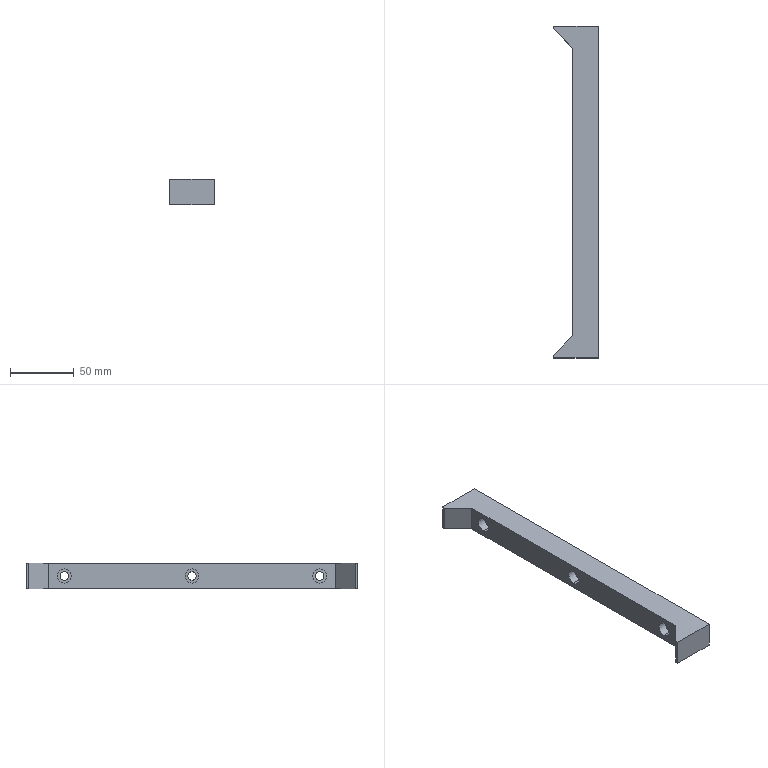Part | STEP file | X77-03204g | 1 solid | 25 faces | box 35 x 260 x 20 mm | volume 106557 mm3 | plane 13 | cylinder 12 | commonest cylinder face diameters 6.6 x6 11 x6
STEP:
#1=CARTESIAN_POINT('',(-11.074,-15.,-15.5));
#2=VERTEX_POINT('',#1);
#3=CARTESIAN_POINT('',(-11.074,-15.,-4.5));
#4=VERTEX_POINT('',#3);
#5=CARTESIAN_POINT('',(-11.074,-15.,-10.));
#6=DIRECTION('',(-1.,0.,0.));
#7=DIRECTION('',(0.,0.,1.));
#8=AXIS2_PLACEMENT_3D('',#5,#6,#7);
#9=CIRCLE('',#8,5.5);
#10=EDGE_CURVE('',#2,#4,#9,.T.);
#11=ORIENTED_EDGE('',*,*,#10,.F.);
#12=CARTESIAN_POINT('',(-17.874,-15.,-15.5));
#13=VERTEX_POINT('',#12);
#14=CARTESIAN_POINT('',(-17.874,-15.,-15.5));
#15=DIRECTION('',(-1.,0.,0.));
#16=VECTOR('',#15,1000.);
#17=LINE('',#14,#16);
#18=EDGE_CURVE('',#2,#13,#17,.T.);
#19=ORIENTED_EDGE('',*,*,#18,.T.);
#20=CARTESIAN_POINT('',(-17.874,-15.,-4.5));
#21=VERTEX_POINT('',#20);
#22=CARTESIAN_POINT('',(-17.874,-15.,-10.));
#23=DIRECTION('',(-1.,0.,0.));
#24=DIRECTION('',(0.,0.,1.));
#25=AXIS2_PLACEMENT_3D('',#22,#23,#24);
#26=CIRCLE('',#25,5.5);
#27=EDGE_CURVE('',#13,#21,#26,.T.);
#28=ORIENTED_EDGE('',*,*,#27,.T.);
#29=CARTESIAN_POINT('',(-17.874,-15.,-4.5));
#30=DIRECTION('',(-1.,0.,0.));
#31=VECTOR('',#30,1000.);
#32=LINE('',#29,#31);
#33=EDGE_CURVE('',#4,#21,#32,.T.);
#34=ORIENTED_EDGE('',*,*,#33,.F.);
#35=EDGE_LOOP('',(#11,#19,#28,#34));
#36=FACE_OUTER_BOUND('',#35,.T.);
#37=CARTESIAN_POINT('',(-17.874,-15.,-10.));
#38=DIRECTION('',(-1.,0.,0.));
#39=DIRECTION('',(0.,0.,1.));
#40=AXIS2_PLACEMENT_3D('',#37,#38,#39);
#41=CYLINDRICAL_SURFACE('',#40,5.5);
#42=ADVANCED_FACE('',(#36),#41,.F.);
#43=CARTESIAN_POINT('',(2.126,-15.,-13.3));
#44=VERTEX_POINT('',#43);
#45=CARTESIAN_POINT('',(2.126,-15.,-6.7));
#46=VERTEX_POINT('',#45);
#47=CARTESIAN_POINT('',(2.126,-15.,-10.));
#48=DIRECTION('',(-1.,0.,0.));
#49=DIRECTION('',(0.,0.,1.));
#50=AXIS2_PLACEMENT_3D('',#47,#48,#49);
#51=CIRCLE('',#50,3.3);
#52=EDGE_CURVE('',#44,#46,#51,.T.);
#53=ORIENTED_EDGE('',*,*,#52,.F.);
#54=CARTESIAN_POINT('',(-11.074,-15.,-13.3));
#55=VERTEX_POINT('',#54);
#56=CARTESIAN_POINT('',(-17.874,-15.,-13.3));
#57=DIRECTION('',(-1.,0.,0.));
#58=VECTOR('',#57,1000.);
#59=LINE('',#56,#58);
#60=EDGE_CURVE('',#44,#55,#59,.T.);
#61=ORIENTED_EDGE('',*,*,#60,.T.);
#62=CARTESIAN_POINT('',(-11.074,-15.,-6.7));
#63=VERTEX_POINT('',#62);
#64=CARTESIAN_POINT('',(-11.074,-15.,-10.));
#65=DIRECTION('',(-1.,0.,0.));
#66=DIRECTION('',(0.,0.,1.));
#67=AXIS2_PLACEMENT_3D('',#64,#65,#66);
#68=CIRCLE('',#67,3.3);
#69=EDGE_CURVE('',#55,#63,#68,.T.);
#70=ORIENTED_EDGE('',*,*,#69,.T.);
#71=CARTESIAN_POINT('',(-17.874,-15.,-6.7));
#72=DIRECTION('',(-1.,0.,0.));
#73=VECTOR('',#72,1000.);
#74=LINE('',#71,#73);
#75=EDGE_CURVE('',#46,#63,#74,.T.);
#76=ORIENTED_EDGE('',*,*,#75,.F.);
#77=EDGE_LOOP('',(#53,#61,#70,#76));
#78=FACE_OUTER_BOUND('',#77,.T.);
#79=CARTESIAN_POINT('',(-17.874,-15.,-10.));
#80=DIRECTION('',(-1.,0.,0.));
#81=DIRECTION('',(0.,0.,1.));
#82=AXIS2_PLACEMENT_3D('',#79,#80,#81);
#83=CYLINDRICAL_SURFACE('',#82,3.3);
#84=ADVANCED_FACE('',(#78),#83,.F.);
#85=CARTESIAN_POINT('',(-11.074,-115.,-15.5));
#86=VERTEX_POINT('',#85);
#87=CARTESIAN_POINT('',(-11.074,-115.,-4.5));
#88=VERTEX_POINT('',#87);
#89=CARTESIAN_POINT('',(-11.074,-115.,-10.));
#90=DIRECTION('',(-1.,0.,0.));
#91=DIRECTION('',(0.,0.,1.));
#92=AXIS2_PLACEMENT_3D('',#89,#90,#91);
#93=CIRCLE('',#92,5.5);
#94=EDGE_CURVE('',#86,#88,#93,.T.);
#95=ORIENTED_EDGE('',*,*,#94,.F.);
#96=CARTESIAN_POINT('',(-17.874,-115.,-15.5));
#97=VERTEX_POINT('',#96);
#98=CARTESIAN_POINT('',(-17.874,-115.,-15.5));
#99=DIRECTION('',(-1.,0.,0.));
#100=VECTOR('',#99,1000.);
#101=LINE('',#98,#100);
#102=EDGE_CURVE('',#86,#97,#101,.T.);
#103=ORIENTED_EDGE('',*,*,#102,.T.);
#104=CARTESIAN_POINT('',(-17.874,-115.,-4.5));
#105=VERTEX_POINT('',#104);
#106=CARTESIAN_POINT('',(-17.874,-115.,-10.));
#107=DIRECTION('',(-1.,0.,0.));
#108=DIRECTION('',(0.,0.,1.));
#109=AXIS2_PLACEMENT_3D('',#106,#107,#108);
#110=CIRCLE('',#109,5.5);
#111=EDGE_CURVE('',#97,#105,#110,.T.);
#112=ORIENTED_EDGE('',*,*,#111,.T.);
#113=CARTESIAN_POINT('',(-17.874,-115.,-4.5));
#114=DIRECTION('',(-1.,0.,0.));
#115=VECTOR('',#114,1000.);
#116=LINE('',#113,#115);
#117=EDGE_CURVE('',#88,#105,#116,.T.);
#118=ORIENTED_EDGE('',*,*,#117,.F.);
#119=EDGE_LOOP('',(#95,#103,#112,#118));
#120=FACE_OUTER_BOUND('',#119,.T.);
#121=CARTESIAN_POINT('',(-17.874,-115.,-10.));
#122=DIRECTION('',(-1.,0.,0.));
#123=DIRECTION('',(0.,0.,1.));
#124=AXIS2_PLACEMENT_3D('',#121,#122,#123);
#125=CYLINDRICAL_SURFACE('',#124,5.5);
#126=ADVANCED_FACE('',(#120),#125,.F.);
#127=CARTESIAN_POINT('',(2.126,-115.,-13.3));
#128=VERTEX_POINT('',#127);
#129=CARTESIAN_POINT('',(2.126,-115.,-6.7));
#130=VERTEX_POINT('',#129);
#131=CARTESIAN_POINT('',(2.126,-115.,-10.));
#132=DIRECTION('',(-1.,0.,0.));
#133=DIRECTION('',(0.,0.,1.));
#134=AXIS2_PLACEMENT_3D('',#131,#132,#133);
#135=CIRCLE('',#134,3.3);
#136=EDGE_CURVE('',#128,#130,#135,.T.);
#137=ORIENTED_EDGE('',*,*,#136,.F.);
#138=CARTESIAN_POINT('',(-11.074,-115.,-13.3));
#139=VERTEX_POINT('',#138);
#140=CARTESIAN_POINT('',(-17.874,-115.,-13.3));
#141=DIRECTION('',(-1.,0.,0.));
#142=VECTOR('',#141,1000.);
#143=LINE('',#140,#142);
#144=EDGE_CURVE('',#128,#139,#143,.T.);
#145=ORIENTED_EDGE('',*,*,#144,.T.);
#146=CARTESIAN_POINT('',(-11.074,-115.,-6.7));
#147=VERTEX_POINT('',#146);
#148=CARTESIAN_POINT('',(-11.074,-115.,-10.));
#149=DIRECTION('',(-1.,0.,0.));
#150=DIRECTION('',(0.,0.,1.));
#151=AXIS2_PLACEMENT_3D('',#148,#149,#150);
#152=CIRCLE('',#151,3.3);
#153=EDGE_CURVE('',#139,#147,#152,.T.);
#154=ORIENTED_EDGE('',*,*,#153,.T.);
#155=CARTESIAN_POINT('',(-17.874,-115.,-6.7));
#156=DIRECTION('',(-1.,0.,0.));
#157=VECTOR('',#156,1000.);
#158=LINE('',#155,#157);
#159=EDGE_CURVE('',#130,#147,#158,.T.);
#160=ORIENTED_EDGE('',*,*,#159,.F.);
#161=EDGE_LOOP('',(#137,#145,#154,#160));
#162=FACE_OUTER_BOUND('',#161,.T.);
#163=CARTESIAN_POINT('',(-17.874,-115.,-10.));
#164=DIRECTION('',(-1.,0.,0.));
#165=DIRECTION('',(0.,0.,1.));
#166=AXIS2_PLACEMENT_3D('',#163,#164,#165);
#167=CYLINDRICAL_SURFACE('',#166,3.3);
#168=ADVANCED_FACE('',(#162),#167,.F.);
#169=CARTESIAN_POINT('',(-11.074,-215.,-15.5));
#170=VERTEX_POINT('',#169);
#171=CARTESIAN_POINT('',(-11.074,-215.,-4.5));
#172=VERTEX_POINT('',#171);
#173=CARTESIAN_POINT('',(-11.074,-215.,-10.));
#174=DIRECTION('',(-1.,0.,0.));
#175=DIRECTION('',(0.,0.,1.));
#176=AXIS2_PLACEMENT_3D('',#173,#174,#175);
#177=CIRCLE('',#176,5.5);
#178=EDGE_CURVE('',#170,#172,#177,.T.);
#179=ORIENTED_EDGE('',*,*,#178,.F.);
#180=CARTESIAN_POINT('',(-17.874,-215.,-15.5));
#181=VERTEX_POINT('',#180);
#182=CARTESIAN_POINT('',(-17.874,-215.,-15.5));
#183=DIRECTION('',(-1.,0.,0.));
#184=VECTOR('',#183,1000.);
#185=LINE('',#182,#184);
#186=EDGE_CURVE('',#170,#181,#185,.T.);
#187=ORIENTED_EDGE('',*,*,#186,.T.);
#188=CARTESIAN_POINT('',(-17.874,-215.,-4.5));
#189=VERTEX_POINT('',#188);
#190=CARTESIAN_POINT('',(-17.874,-215.,-10.));
#191=DIRECTION('',(-1.,0.,0.));
#192=DIRECTION('',(0.,0.,1.));
#193=AXIS2_PLACEMENT_3D('',#190,#191,#192);
#194=CIRCLE('',#193,5.5);
#195=EDGE_CURVE('',#181,#189,#194,.T.);
#196=ORIENTED_EDGE('',*,*,#195,.T.);
#197=CARTESIAN_POINT('',(-17.874,-215.,-4.5));
#198=DIRECTION('',(-1.,0.,0.));
#199=VECTOR('',#198,1000.);
#200=LINE('',#197,#199);
#201=EDGE_CURVE('',#172,#189,#200,.T.);
#202=ORIENTED_EDGE('',*,*,#201,.F.);
#203=EDGE_LOOP('',(#179,#187,#196,#202));
#204=FACE_OUTER_BOUND('',#203,.T.);
#205=CARTESIAN_POINT('',(-17.874,-215.,-10.));
#206=DIRECTION('',(-1.,0.,0.));
#207=DIRECTION('',(0.,0.,1.));
#208=AXIS2_PLACEMENT_3D('',#205,#206,#207);
#209=CYLINDRICAL_SURFACE('',#208,5.5);
#210=ADVANCED_FACE('',(#204),#209,.F.);
#211=CARTESIAN_POINT('',(2.126,-215.,-13.3));
#212=VERTEX_POINT('',#211);
#213=CARTESIAN_POINT('',(2.126,-215.,-6.7));
#214=VERTEX_POINT('',#213);
#215=CARTESIAN_POINT('',(2.126,-215.,-10.));
#216=DIRECTION('',(-1.,0.,0.));
#217=DIRECTION('',(0.,0.,1.));
#218=AXIS2_PLACEMENT_3D('',#215,#216,#217);
#219=CIRCLE('',#218,3.3);
#220=EDGE_CURVE('',#212,#214,#219,.T.);
#221=ORIENTED_EDGE('',*,*,#220,.F.);
#222=CARTESIAN_POINT('',(-11.074,-215.,-13.3));
#223=VERTEX_POINT('',#222);
#224=CARTESIAN_POINT('',(-17.874,-215.,-13.3));
#225=DIRECTION('',(-1.,0.,0.));
#226=VECTOR('',#225,1000.);
#227=LINE('',#224,#226);
#228=EDGE_CURVE('',#212,#223,#227,.T.);
#229=ORIENTED_EDGE('',*,*,#228,.T.);
#230=CARTESIAN_POINT('',(-11.074,-215.,-6.7));
#231=VERTEX_POINT('',#230);
#232=CARTESIAN_POINT('',(-11.074,-215.,-10.));
#233=DIRECTION('',(-1.,0.,0.));
#234=DIRECTION('',(0.,0.,1.));
#235=AXIS2_PLACEMENT_3D('',#232,#233,#234);
#236=CIRCLE('',#235,3.3);
#237=EDGE_CURVE('',#223,#231,#236,.T.);
#238=ORIENTED_EDGE('',*,*,#237,.T.);
#239=CARTESIAN_POINT('',(-17.874,-215.,-6.7));
#240=DIRECTION('',(-1.,0.,0.));
#241=VECTOR('',#240,1000.);
#242=LINE('',#239,#241);
#243=EDGE_CURVE('',#214,#231,#242,.T.);
#244=ORIENTED_EDGE('',*,*,#243,.F.);
#245=EDGE_LOOP('',(#221,#229,#238,#244));
#246=FACE_OUTER_BOUND('',#245,.T.);
#247=CARTESIAN_POINT('',(-17.874,-215.,-10.));
#248=DIRECTION('',(-1.,0.,0.));
#249=DIRECTION('',(0.,0.,1.));
#250=AXIS2_PLACEMENT_3D('',#247,#248,#249);
#251=CYLINDRICAL_SURFACE('',#250,3.3);
#252=ADVANCED_FACE('',(#246),#251,.F.);
#253=CARTESIAN_POINT('',(-17.874,-15.,-10.));
#254=DIRECTION('',(-1.,0.,0.));
#255=DIRECTION('',(0.,0.,1.));
#256=AXIS2_PLACEMENT_3D('',#253,#254,#255);
#257=CIRCLE('',#256,5.5);
#258=EDGE_CURVE('',#21,#13,#257,.T.);
#259=ORIENTED_EDGE('',*,*,#258,.F.);
#260=ORIENTED_EDGE('',*,*,#27,.F.);
#261=EDGE_LOOP('',(#259,#260));
#262=FACE_BOUND('',#261,.T.);
#263=CARTESIAN_POINT('',(-17.874,-115.,-10.));
#264=DIRECTION('',(-1.,0.,0.));
#265=DIRECTION('',(0.,0.,1.));
#266=AXIS2_PLACEMENT_3D('',#263,#264,#265);
#267=CIRCLE('',#266,5.5);
#268=EDGE_CURVE('',#105,#97,#267,.T.);
#269=ORIENTED_EDGE('',*,*,#268,.F.);
#270=ORIENTED_EDGE('',*,*,#111,.F.);
#271=EDGE_LOOP('',(#269,#270));
#272=FACE_BOUND('',#271,.T.);
#273=CARTESIAN_POINT('',(-17.874,-215.,-10.));
#274=DIRECTION('',(-1.,0.,0.));
#275=DIRECTION('',(0.,0.,1.));
#276=AXIS2_PLACEMENT_3D('',#273,#274,#275);
#277=CIRCLE('',#276,5.5);
#278=EDGE_CURVE('',#189,#181,#277,.T.);
#279=ORIENTED_EDGE('',*,*,#278,.F.);
#280=ORIENTED_EDGE('',*,*,#195,.F.);
#281=EDGE_LOOP('',(#279,#280));
#282=FACE_BOUND('',#281,.T.);
#283=CARTESIAN_POINT('',(-17.874,-2.251,0.));
#284=VERTEX_POINT('',#283);
#285=CARTESIAN_POINT('',(-17.874,-227.749,0.));
#286=VERTEX_POINT('',#285);
#287=CARTESIAN_POINT('',(-17.874,-227.749,0.));
#288=DIRECTION('',(0.,-1.,0.));
#289=VECTOR('',#288,1000.);
#290=LINE('',#287,#289);
#291=EDGE_CURVE('',#284,#286,#290,.T.);
#292=ORIENTED_EDGE('',*,*,#291,.F.);
#293=CARTESIAN_POINT('',(-17.874,-2.251,-20.));
#294=VERTEX_POINT('',#293);
#295=CARTESIAN_POINT('',(-17.874,-2.251,-20.));
#296=DIRECTION('',(0.,0.,1.));
#297=VECTOR('',#296,1000.);
#298=LINE('',#295,#297);
#299=EDGE_CURVE('',#294,#284,#298,.T.);
#300=ORIENTED_EDGE('',*,*,#299,.F.);
#301=CARTESIAN_POINT('',(-17.874,-227.749,-20.));
#302=VERTEX_POINT('',#301);
#303=CARTESIAN_POINT('',(-17.874,-227.749,-20.));
#304=DIRECTION('',(0.,-1.,0.));
#305=VECTOR('',#304,1000.);
#306=LINE('',#303,#305);
#307=EDGE_CURVE('',#294,#302,#306,.T.);
#308=ORIENTED_EDGE('',*,*,#307,.T.);
#309=CARTESIAN_POINT('',(-17.874,-227.749,-20.));
#310=DIRECTION('',(0.,0.,1.));
#311=VECTOR('',#310,1000.);
#312=LINE('',#309,#311);
#313=EDGE_CURVE('',#302,#286,#312,.T.);
#314=ORIENTED_EDGE('',*,*,#313,.T.);
#315=EDGE_LOOP('',(#292,#300,#308,#314));
#316=FACE_OUTER_BOUND('',#315,.T.);
#317=CARTESIAN_POINT('',(-17.874,-227.749,-20.));
#318=DIRECTION('',(-1.,0.,0.));
#319=DIRECTION('',(0.,-1.,0.));
#320=AXIS2_PLACEMENT_3D('',#317,#318,#319);
#321=PLANE('',#320);
#322=ADVANCED_FACE('',(#262,#272,#282,#316),#321,.T.);
#323=CARTESIAN_POINT('',(-32.874,12.749,0.));
#324=VERTEX_POINT('',#323);
#325=CARTESIAN_POINT('',(-17.874,-2.251,0.));
#326=DIRECTION('',(0.7071,-0.7071,0.));
#327=VECTOR('',#326,1000.);
#328=LINE('',#325,#327);
#329=EDGE_CURVE('',#324,#284,#328,.T.);
#330=ORIENTED_EDGE('',*,*,#329,.F.);
#331=CARTESIAN_POINT('',(-32.874,12.749,-20.));
#332=VERTEX_POINT('',#331);
#333=CARTESIAN_POINT('',(-32.874,12.749,-20.));
#334=DIRECTION('',(0.,0.,1.));
#335=VECTOR('',#334,1000.);
#336=LINE('',#333,#335);
#337=EDGE_CURVE('',#332,#324,#336,.T.);
#338=ORIENTED_EDGE('',*,*,#337,.F.);
#339=CARTESIAN_POINT('',(-17.874,-2.251,-20.));
#340=DIRECTION('',(0.7071,-0.7071,0.));
#341=VECTOR('',#340,1000.);
#342=LINE('',#339,#341);
#343=EDGE_CURVE('',#332,#294,#342,.T.);
#344=ORIENTED_EDGE('',*,*,#343,.T.);
#345=ORIENTED_EDGE('',*,*,#299,.T.);
#346=EDGE_LOOP('',(#330,#338,#344,#345));
#347=FACE_OUTER_BOUND('',#346,.T.);
#348=CARTESIAN_POINT('',(-17.874,-2.251,-20.));
#349=DIRECTION('',(-0.7071,-0.7071,0.));
#350=DIRECTION('',(0.7071,-0.7071,0.));
#351=AXIS2_PLACEMENT_3D('',#348,#349,#350);
#352=PLANE('',#351);
#353=ADVANCED_FACE('',(#347),#352,.T.);
#354=CARTESIAN_POINT('',(-32.874,15.,0.));
#355=VERTEX_POINT('',#354);
#356=CARTESIAN_POINT('',(-32.874,12.749,0.));
#357=DIRECTION('',(0.,-1.,0.));
#358=VECTOR('',#357,1000.);
#359=LINE('',#356,#358);
#360=EDGE_CURVE('',#355,#324,#359,.T.);
#361=ORIENTED_EDGE('',*,*,#360,.F.);
#362=CARTESIAN_POINT('',(-32.874,15.,-20.));
#363=VERTEX_POINT('',#362);
#364=CARTESIAN_POINT('',(-32.874,15.,-20.));
#365=DIRECTION('',(0.,0.,1.));
#366=VECTOR('',#365,1000.);
#367=LINE('',#364,#366);
#368=EDGE_CURVE('',#363,#355,#367,.T.);
#369=ORIENTED_EDGE('',*,*,#368,.F.);
#370=CARTESIAN_POINT('',(-32.874,12.749,-20.));
#371=DIRECTION('',(0.,-1.,0.));
#372=VECTOR('',#371,1000.);
#373=LINE('',#370,#372);
#374=EDGE_CURVE('',#363,#332,#373,.T.);
#375=ORIENTED_EDGE('',*,*,#374,.T.);
#376=ORIENTED_EDGE('',*,*,#337,.T.);
#377=EDGE_LOOP('',(#361,#369,#375,#376));
#378=FACE_OUTER_BOUND('',#377,.T.);
#379=CARTESIAN_POINT('',(-32.874,12.749,-20.));
#380=DIRECTION('',(-1.,0.,0.));
#381=DIRECTION('',(0.,0.,1.));
#382=AXIS2_PLACEMENT_3D('',#379,#380,#381);
#383=PLANE('',#382);
#384=ADVANCED_FACE('',(#378),#383,.T.);
#385=CARTESIAN_POINT('',(2.126,15.,0.));
#386=VERTEX_POINT('',#385);
#387=CARTESIAN_POINT('',(2.126,15.,0.));
#388=DIRECTION('',(-1.,0.,0.));
#389=VECTOR('',#388,1000.);
#390=LINE('',#387,#389);
#391=EDGE_CURVE('',#386,#355,#390,.T.);
#392=ORIENTED_EDGE('',*,*,#391,.F.);
#393=CARTESIAN_POINT('',(2.126,15.,-20.));
#394=VERTEX_POINT('',#393);
#395=CARTESIAN_POINT('',(2.126,15.,-20.));
#396=DIRECTION('',(0.,0.,1.));
#397=VECTOR('',#396,1000.);
#398=LINE('',#395,#397);
#399=EDGE_CURVE('',#394,#386,#398,.T.);
#400=ORIENTED_EDGE('',*,*,#399,.F.);
#401=CARTESIAN_POINT('',(2.126,15.,-20.));
#402=DIRECTION('',(-1.,0.,0.));
#403=VECTOR('',#402,1000.);
#404=LINE('',#401,#403);
#405=EDGE_CURVE('',#394,#363,#404,.T.);
#406=ORIENTED_EDGE('',*,*,#405,.T.);
#407=ORIENTED_EDGE('',*,*,#368,.T.);
#408=EDGE_LOOP('',(#392,#400,#406,#407));
#409=FACE_OUTER_BOUND('',#408,.T.);
#410=CARTESIAN_POINT('',(2.126,15.,-20.));
#411=DIRECTION('',(0.,1.,0.));
#412=DIRECTION('',(0.,0.,1.));
#413=AXIS2_PLACEMENT_3D('',#410,#411,#412);
#414=PLANE('',#413);
#415=ADVANCED_FACE('',(#409),#414,.T.);
#416=CARTESIAN_POINT('',(2.126,-15.,-10.));
#417=DIRECTION('',(-1.,0.,0.));
#418=DIRECTION('',(0.,0.,1.));
#419=AXIS2_PLACEMENT_3D('',#416,#417,#418);
#420=CIRCLE('',#419,3.3);
#421=EDGE_CURVE('',#46,#44,#420,.T.);
#422=ORIENTED_EDGE('',*,*,#421,.T.);
#423=ORIENTED_EDGE('',*,*,#52,.T.);
#424=EDGE_LOOP('',(#422,#423));
#425=FACE_BOUND('',#424,.T.);
#426=CARTESIAN_POINT('',(2.126,-115.,-10.));
#427=DIRECTION('',(-1.,0.,0.));
#428=DIRECTION('',(0.,0.,1.));
#429=AXIS2_PLACEMENT_3D('',#426,#427,#428);
#430=CIRCLE('',#429,3.3);
#431=EDGE_CURVE('',#130,#128,#430,.T.);
#432=ORIENTED_EDGE('',*,*,#431,.T.);
#433=ORIENTED_EDGE('',*,*,#136,.T.);
#434=EDGE_LOOP('',(#432,#433));
#435=FACE_BOUND('',#434,.T.);
#436=CARTESIAN_POINT('',(2.126,-215.,-10.));
#437=DIRECTION('',(-1.,0.,0.));
#438=DIRECTION('',(0.,0.,1.));
#439=AXIS2_PLACEMENT_3D('',#436,#437,#438);
#440=CIRCLE('',#439,3.3);
#441=EDGE_CURVE('',#214,#212,#440,.T.);
#442=ORIENTED_EDGE('',*,*,#441,.T.);
#443=ORIENTED_EDGE('',*,*,#220,.T.);
#444=EDGE_LOOP('',(#442,#443));
#445=FACE_BOUND('',#444,.T.);
#446=CARTESIAN_POINT('',(2.126,-245.,0.));
#447=VERTEX_POINT('',#446);
#448=CARTESIAN_POINT('',(2.126,-245.,0.));
#449=DIRECTION('',(0.,1.,0.));
#450=VECTOR('',#449,1000.);
#451=LINE('',#448,#450);
#452=EDGE_CURVE('',#447,#386,#451,.T.);
#453=ORIENTED_EDGE('',*,*,#452,.F.);
#454=CARTESIAN_POINT('',(2.126,-245.,-20.));
#455=VERTEX_POINT('',#454);
#456=CARTESIAN_POINT('',(2.126,-245.,-20.));
#457=DIRECTION('',(0.,0.,1.));
#458=VECTOR('',#457,1000.);
#459=LINE('',#456,#458);
#460=EDGE_CURVE('',#455,#447,#459,.T.);
#461=ORIENTED_EDGE('',*,*,#460,.F.);
#462=CARTESIAN_POINT('',(2.126,-245.,-20.));
#463=DIRECTION('',(0.,1.,0.));
#464=VECTOR('',#463,1000.);
#465=LINE('',#462,#464);
#466=EDGE_CURVE('',#455,#394,#465,.T.);
#467=ORIENTED_EDGE('',*,*,#466,.T.);
#468=ORIENTED_EDGE('',*,*,#399,.T.);
#469=EDGE_LOOP('',(#453,#461,#467,#468));
#470=FACE_OUTER_BOUND('',#469,.T.);
#471=CARTESIAN_POINT('',(2.126,-245.,-20.));
#472=DIRECTION('',(1.,0.,0.));
#473=DIRECTION('',(0.,1.,0.));
#474=AXIS2_PLACEMENT_3D('',#471,#472,#473);
#475=PLANE('',#474);
#476=ADVANCED_FACE('',(#425,#435,#445,#470),#475,.T.);
#477=CARTESIAN_POINT('',(-32.874,-245.,0.));
#478=VERTEX_POINT('',#477);
#479=CARTESIAN_POINT('',(2.126,-245.,0.));
#480=DIRECTION('',(1.,0.,0.));
#481=VECTOR('',#480,1000.);
#482=LINE('',#479,#481);
#483=EDGE_CURVE('',#478,#447,#482,.T.);
#484=ORIENTED_EDGE('',*,*,#483,.F.);
#485=CARTESIAN_POINT('',(-32.874,-245.,-20.));
#486=VERTEX_POINT('',#485);
#487=CARTESIAN_POINT('',(-32.874,-245.,-20.));
#488=DIRECTION('',(0.,0.,1.));
#489=VECTOR('',#488,1000.);
#490=LINE('',#487,#489);
#491=EDGE_CURVE('',#486,#478,#490,.T.);
#492=ORIENTED_EDGE('',*,*,#491,.F.);
#493=CARTESIAN_POINT('',(2.126,-245.,-20.));
#494=DIRECTION('',(1.,0.,0.));
#495=VECTOR('',#494,1000.);
#496=LINE('',#493,#495);
#497=EDGE_CURVE('',#486,#455,#496,.T.);
#498=ORIENTED_EDGE('',*,*,#497,.T.);
#499=ORIENTED_EDGE('',*,*,#460,.T.);
#500=EDGE_LOOP('',(#484,#492,#498,#499));
#501=FACE_OUTER_BOUND('',#500,.T.);
#502=CARTESIAN_POINT('',(2.126,-245.,-20.));
#503=DIRECTION('',(0.,-1.,0.));
#504=DIRECTION('',(0.,0.,-1.));
#505=AXIS2_PLACEMENT_3D('',#502,#503,#504);
#506=PLANE('',#505);
#507=ADVANCED_FACE('',(#501),#506,.T.);
#508=CARTESIAN_POINT('',(-32.874,-242.749,0.));
#509=VERTEX_POINT('',#508);
#510=CARTESIAN_POINT('',(-32.874,-242.749,0.));
#511=DIRECTION('',(0.,-1.,0.));
#512=VECTOR('',#511,1000.);
#513=LINE('',#510,#512);
#514=EDGE_CURVE('',#509,#478,#513,.T.);
#515=ORIENTED_EDGE('',*,*,#514,.F.);
#516=CARTESIAN_POINT('',(-32.874,-242.749,-20.));
#517=VERTEX_POINT('',#516);
#518=CARTESIAN_POINT('',(-32.874,-242.749,-20.));
#519=DIRECTION('',(0.,0.,1.));
#520=VECTOR('',#519,1000.);
#521=LINE('',#518,#520);
#522=EDGE_CURVE('',#517,#509,#521,.T.);
#523=ORIENTED_EDGE('',*,*,#522,.F.);
#524=CARTESIAN_POINT('',(-32.874,-242.749,-20.));
#525=DIRECTION('',(0.,-1.,0.));
#526=VECTOR('',#525,1000.);
#527=LINE('',#524,#526);
#528=EDGE_CURVE('',#517,#486,#527,.T.);
#529=ORIENTED_EDGE('',*,*,#528,.T.);
#530=ORIENTED_EDGE('',*,*,#491,.T.);
#531=EDGE_LOOP('',(#515,#523,#529,#530));
#532=FACE_OUTER_BOUND('',#531,.T.);
#533=CARTESIAN_POINT('',(-32.874,-242.749,-20.));
#534=DIRECTION('',(-1.,0.,0.));
#535=DIRECTION('',(0.,0.,1.));
#536=AXIS2_PLACEMENT_3D('',#533,#534,#535);
#537=PLANE('',#536);
#538=ADVANCED_FACE('',(#532),#537,.T.);
#539=CARTESIAN_POINT('',(-17.874,-227.749,0.));
#540=DIRECTION('',(-0.7071,-0.7071,0.));
#541=VECTOR('',#540,1000.);
#542=LINE('',#539,#541);
#543=EDGE_CURVE('',#286,#509,#542,.T.);
#544=ORIENTED_EDGE('',*,*,#543,.F.);
#545=ORIENTED_EDGE('',*,*,#313,.F.);
#546=CARTESIAN_POINT('',(-17.874,-227.749,-20.));
#547=DIRECTION('',(-0.7071,-0.7071,0.));
#548=VECTOR('',#547,1000.);
#549=LINE('',#546,#548);
#550=EDGE_CURVE('',#302,#517,#549,.T.);
#551=ORIENTED_EDGE('',*,*,#550,.T.);
#552=ORIENTED_EDGE('',*,*,#522,.T.);
#553=EDGE_LOOP('',(#544,#545,#551,#552));
#554=FACE_OUTER_BOUND('',#553,.T.);
#555=CARTESIAN_POINT('',(-17.874,-227.749,-20.));
#556=DIRECTION('',(-0.7071,0.7071,0.));
#557=DIRECTION('',(-0.7071,-0.7071,0.));
#558=AXIS2_PLACEMENT_3D('',#555,#556,#557);
#559=PLANE('',#558);
#560=ADVANCED_FACE('',(#554),#559,.T.);
#561=ORIENTED_EDGE('',*,*,#307,.F.);
#562=ORIENTED_EDGE('',*,*,#343,.F.);
#563=ORIENTED_EDGE('',*,*,#374,.F.);
#564=ORIENTED_EDGE('',*,*,#405,.F.);
#565=ORIENTED_EDGE('',*,*,#466,.F.);
#566=ORIENTED_EDGE('',*,*,#497,.F.);
#567=ORIENTED_EDGE('',*,*,#528,.F.);
#568=ORIENTED_EDGE('',*,*,#550,.F.);
#569=EDGE_LOOP('',(#561,#562,#563,#564,#565,#566,#567,#568));
#570=FACE_OUTER_BOUND('',#569,.T.);
#571=CARTESIAN_POINT('',(-17.874,15.,-20.));
#572=DIRECTION('',(0.,0.,1.));
#573=DIRECTION('',(1.,0.,0.));
#574=AXIS2_PLACEMENT_3D('',#571,#572,#573);
#575=PLANE('',#574);
#576=ADVANCED_FACE('',(#570),#575,.F.);
#577=ORIENTED_EDGE('',*,*,#291,.T.);
#578=ORIENTED_EDGE('',*,*,#543,.T.);
#579=ORIENTED_EDGE('',*,*,#514,.T.);
#580=ORIENTED_EDGE('',*,*,#483,.T.);
#581=ORIENTED_EDGE('',*,*,#452,.T.);
#582=ORIENTED_EDGE('',*,*,#391,.T.);
#583=ORIENTED_EDGE('',*,*,#360,.T.);
#584=ORIENTED_EDGE('',*,*,#329,.T.);
#585=EDGE_LOOP('',(#577,#578,#579,#580,#581,#582,#583,#584));
#586=FACE_OUTER_BOUND('',#585,.T.);
#587=CARTESIAN_POINT('',(-17.874,15.,0.));
#588=DIRECTION('',(0.,0.,1.));
#589=DIRECTION('',(1.,0.,0.));
#590=AXIS2_PLACEMENT_3D('',#587,#588,#589);
#591=PLANE('',#590);
#592=ADVANCED_FACE('',(#586),#591,.T.);
#593=ORIENTED_EDGE('',*,*,#228,.F.);
#594=ORIENTED_EDGE('',*,*,#441,.F.);
#595=ORIENTED_EDGE('',*,*,#243,.T.);
#596=CARTESIAN_POINT('',(-11.074,-215.,-10.));
#597=DIRECTION('',(-1.,0.,0.));
#598=DIRECTION('',(0.,0.,1.));
#599=AXIS2_PLACEMENT_3D('',#596,#597,#598);
#600=CIRCLE('',#599,3.3);
#601=EDGE_CURVE('',#231,#223,#600,.T.);
#602=ORIENTED_EDGE('',*,*,#601,.T.);
#603=EDGE_LOOP('',(#593,#594,#595,#602));
#604=FACE_OUTER_BOUND('',#603,.T.);
#605=CARTESIAN_POINT('',(-17.874,-215.,-10.));
#606=DIRECTION('',(-1.,0.,0.));
#607=DIRECTION('',(0.,0.,1.));
#608=AXIS2_PLACEMENT_3D('',#605,#606,#607);
#609=CYLINDRICAL_SURFACE('',#608,3.3);
#610=ADVANCED_FACE('',(#604),#609,.F.);
#611=ORIENTED_EDGE('',*,*,#601,.F.);
#612=ORIENTED_EDGE('',*,*,#237,.F.);
#613=EDGE_LOOP('',(#611,#612));
#614=FACE_BOUND('',#613,.T.);
#615=CARTESIAN_POINT('',(-11.074,-215.,-10.));
#616=DIRECTION('',(-1.,0.,0.));
#617=DIRECTION('',(0.,0.,1.));
#618=AXIS2_PLACEMENT_3D('',#615,#616,#617);
#619=CIRCLE('',#618,5.5);
#620=EDGE_CURVE('',#172,#170,#619,.T.);
#621=ORIENTED_EDGE('',*,*,#620,.T.);
#622=ORIENTED_EDGE('',*,*,#178,.T.);
#623=EDGE_LOOP('',(#621,#622));
#624=FACE_OUTER_BOUND('',#623,.T.);
#625=CARTESIAN_POINT('',(-11.074,-211.7,-10.));
#626=DIRECTION('',(1.,0.,0.));
#627=DIRECTION('',(0.,0.,-1.));
#628=AXIS2_PLACEMENT_3D('',#625,#626,#627);
#629=PLANE('',#628);
#630=ADVANCED_FACE('',(#614,#624),#629,.F.);
#631=ORIENTED_EDGE('',*,*,#186,.F.);
#632=ORIENTED_EDGE('',*,*,#620,.F.);
#633=ORIENTED_EDGE('',*,*,#201,.T.);
#634=ORIENTED_EDGE('',*,*,#278,.T.);
#635=EDGE_LOOP('',(#631,#632,#633,#634));
#636=FACE_OUTER_BOUND('',#635,.T.);
#637=CARTESIAN_POINT('',(-17.874,-215.,-10.));
#638=DIRECTION('',(-1.,0.,0.));
#639=DIRECTION('',(0.,0.,1.));
#640=AXIS2_PLACEMENT_3D('',#637,#638,#639);
#641=CYLINDRICAL_SURFACE('',#640,5.5);
#642=ADVANCED_FACE('',(#636),#641,.F.);
#643=ORIENTED_EDGE('',*,*,#144,.F.);
#644=ORIENTED_EDGE('',*,*,#431,.F.);
#645=ORIENTED_EDGE('',*,*,#159,.T.);
#646=CARTESIAN_POINT('',(-11.074,-115.,-10.));
#647=DIRECTION('',(-1.,0.,0.));
#648=DIRECTION('',(0.,0.,1.));
#649=AXIS2_PLACEMENT_3D('',#646,#647,#648);
#650=CIRCLE('',#649,3.3);
#651=EDGE_CURVE('',#147,#139,#650,.T.);
#652=ORIENTED_EDGE('',*,*,#651,.T.);
#653=EDGE_LOOP('',(#643,#644,#645,#652));
#654=FACE_OUTER_BOUND('',#653,.T.);
#655=CARTESIAN_POINT('',(-17.874,-115.,-10.));
#656=DIRECTION('',(-1.,0.,0.));
#657=DIRECTION('',(0.,0.,1.));
#658=AXIS2_PLACEMENT_3D('',#655,#656,#657);
#659=CYLINDRICAL_SURFACE('',#658,3.3);
#660=ADVANCED_FACE('',(#654),#659,.F.);
#661=ORIENTED_EDGE('',*,*,#651,.F.);
#662=ORIENTED_EDGE('',*,*,#153,.F.);
#663=EDGE_LOOP('',(#661,#662));
#664=FACE_BOUND('',#663,.T.);
#665=CARTESIAN_POINT('',(-11.074,-115.,-10.));
#666=DIRECTION('',(-1.,0.,0.));
#667=DIRECTION('',(0.,0.,1.));
#668=AXIS2_PLACEMENT_3D('',#665,#666,#667);
#669=CIRCLE('',#668,5.5);
#670=EDGE_CURVE('',#88,#86,#669,.T.);
#671=ORIENTED_EDGE('',*,*,#670,.T.);
#672=ORIENTED_EDGE('',*,*,#94,.T.);
#673=EDGE_LOOP('',(#671,#672));
#674=FACE_OUTER_BOUND('',#673,.T.);
#675=CARTESIAN_POINT('',(-11.074,-111.7,-10.));
#676=DIRECTION('',(1.,0.,0.));
#677=DIRECTION('',(0.,0.,-1.));
#678=AXIS2_PLACEMENT_3D('',#675,#676,#677);
#679=PLANE('',#678);
#680=ADVANCED_FACE('',(#664,#674),#679,.F.);
#681=ORIENTED_EDGE('',*,*,#102,.F.);
#682=ORIENTED_EDGE('',*,*,#670,.F.);
#683=ORIENTED_EDGE('',*,*,#117,.T.);
#684=ORIENTED_EDGE('',*,*,#268,.T.);
#685=EDGE_LOOP('',(#681,#682,#683,#684));
#686=FACE_OUTER_BOUND('',#685,.T.);
#687=CARTESIAN_POINT('',(-17.874,-115.,-10.));
#688=DIRECTION('',(-1.,0.,0.));
#689=DIRECTION('',(0.,0.,1.));
#690=AXIS2_PLACEMENT_3D('',#687,#688,#689);
#691=CYLINDRICAL_SURFACE('',#690,5.5);
#692=ADVANCED_FACE('',(#686),#691,.F.);
#693=ORIENTED_EDGE('',*,*,#60,.F.);
#694=ORIENTED_EDGE('',*,*,#421,.F.);
#695=ORIENTED_EDGE('',*,*,#75,.T.);
#696=CARTESIAN_POINT('',(-11.074,-15.,-10.));
#697=DIRECTION('',(-1.,0.,0.));
#698=DIRECTION('',(0.,0.,1.));
#699=AXIS2_PLACEMENT_3D('',#696,#697,#698);
#700=CIRCLE('',#699,3.3);
#701=EDGE_CURVE('',#63,#55,#700,.T.);
#702=ORIENTED_EDGE('',*,*,#701,.T.);
#703=EDGE_LOOP('',(#693,#694,#695,#702));
#704=FACE_OUTER_BOUND('',#703,.T.);
#705=CARTESIAN_POINT('',(-17.874,-15.,-10.));
#706=DIRECTION('',(-1.,0.,0.));
#707=DIRECTION('',(0.,0.,1.));
#708=AXIS2_PLACEMENT_3D('',#705,#706,#707);
#709=CYLINDRICAL_SURFACE('',#708,3.3);
#710=ADVANCED_FACE('',(#704),#709,.F.);
#711=ORIENTED_EDGE('',*,*,#701,.F.);
#712=ORIENTED_EDGE('',*,*,#69,.F.);
#713=EDGE_LOOP('',(#711,#712));
#714=FACE_BOUND('',#713,.T.);
#715=CARTESIAN_POINT('',(-11.074,-15.,-10.));
#716=DIRECTION('',(-1.,0.,0.));
#717=DIRECTION('',(0.,0.,1.));
#718=AXIS2_PLACEMENT_3D('',#715,#716,#717);
#719=CIRCLE('',#718,5.5);
#720=EDGE_CURVE('',#4,#2,#719,.T.);
#721=ORIENTED_EDGE('',*,*,#720,.T.);
#722=ORIENTED_EDGE('',*,*,#10,.T.);
#723=EDGE_LOOP('',(#721,#722));
#724=FACE_OUTER_BOUND('',#723,.T.);
#725=CARTESIAN_POINT('',(-11.074,-11.7,-10.));
#726=DIRECTION('',(1.,0.,0.));
#727=DIRECTION('',(0.,0.,-1.));
#728=AXIS2_PLACEMENT_3D('',#725,#726,#727);
#729=PLANE('',#728);
#730=ADVANCED_FACE('',(#714,#724),#729,.F.);
#731=ORIENTED_EDGE('',*,*,#18,.F.);
#732=ORIENTED_EDGE('',*,*,#720,.F.);
#733=ORIENTED_EDGE('',*,*,#33,.T.);
#734=ORIENTED_EDGE('',*,*,#258,.T.);
#735=EDGE_LOOP('',(#731,#732,#733,#734));
#736=FACE_OUTER_BOUND('',#735,.T.);
#737=CARTESIAN_POINT('',(-17.874,-15.,-10.));
#738=DIRECTION('',(-1.,0.,0.));
#739=DIRECTION('',(0.,0.,1.));
#740=AXIS2_PLACEMENT_3D('',#737,#738,#739);
#741=CYLINDRICAL_SURFACE('',#740,5.5);
#742=ADVANCED_FACE('',(#736),#741,.F.);
#743=CLOSED_SHELL('',(#42,#84,#126,#168,#210,#252,#322,#353,#384,#415,#476,#507,#538,#560,#576,#592,#610,#630,#642,#660,#680,#692,#710,#730,#742));
#744=MANIFOLD_SOLID_BREP('',#743);
#745=CARTESIAN_POINT('',(0.,0.,0.));
#746=DIRECTION('',(0.,0.,1.));
#747=DIRECTION('',(1.,0.,0.));
#748=AXIS2_PLACEMENT_3D('',#745,#746,#747);
#749=(LENGTH_UNIT()NAMED_UNIT(*)SI_UNIT(.MILLI.,.METRE.));
#750=UNCERTAINTY_MEASURE_WITH_UNIT(LENGTH_MEASURE(0.00001),#749,'','');
#751=(NAMED_UNIT(*)PLANE_ANGLE_UNIT()SI_UNIT($,.RADIAN.));
#752=(NAMED_UNIT(*)SI_UNIT($,.STERADIAN.)SOLID_ANGLE_UNIT());
#753=(GEOMETRIC_REPRESENTATION_CONTEXT(3)GLOBAL_UNCERTAINTY_ASSIGNED_CONTEXT((#750))GLOBAL_UNIT_ASSIGNED_CONTEXT((#749,#751,#752))REPRESENTATION_CONTEXT('',''));
#754=ADVANCED_BREP_SHAPE_REPRESENTATION('',(#744,#748),#753);